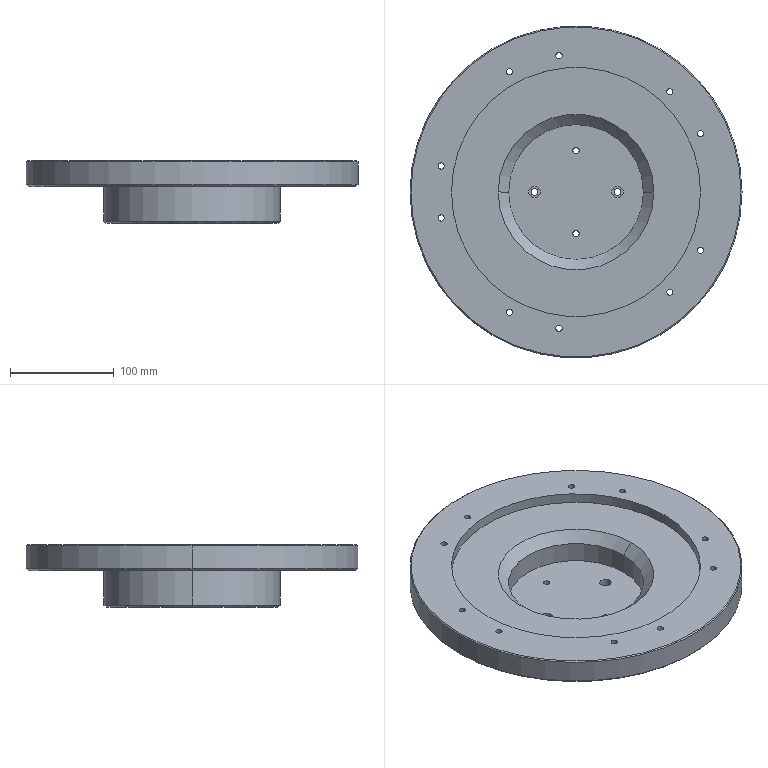Part | 1 solid | 55 faces | box 320 x 320 x 60 mm | volume 1919037 mm3 | cylinder 40 | cone 8 | plane 7 | commonest cylinder face diameters 6 x24 6.6 x4 11 x4 130 x2 170 x2 240 x2